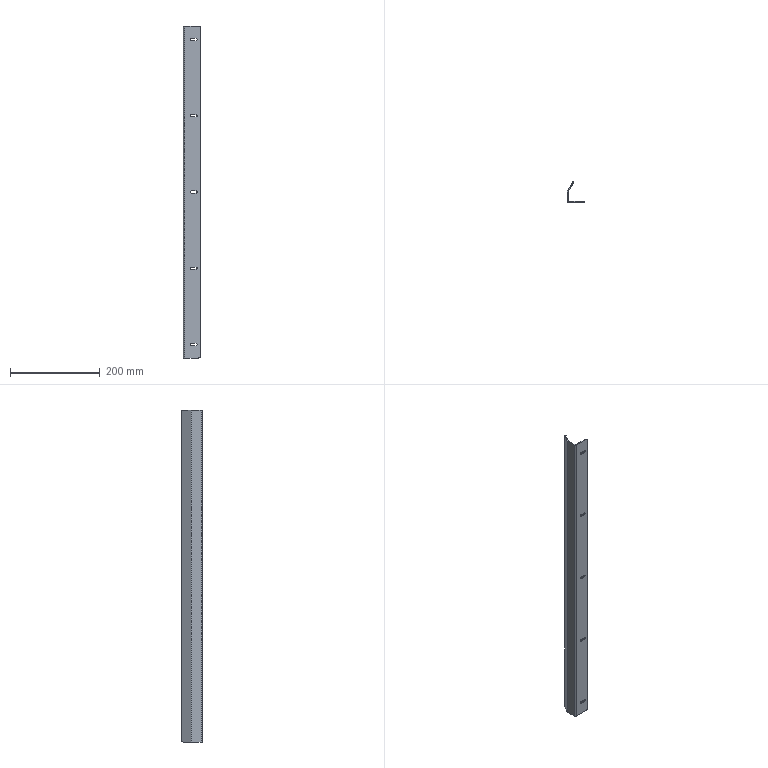Part | STEP file | 0228_211_Guide | 1 solid | 41 faces | box 38 x 46.651 x 740 mm | volume 124477 mm3 | cylinder 21 | plane 20 | commonest cylinder face diameters 5 x15 10 x4 2 x1 6 x1